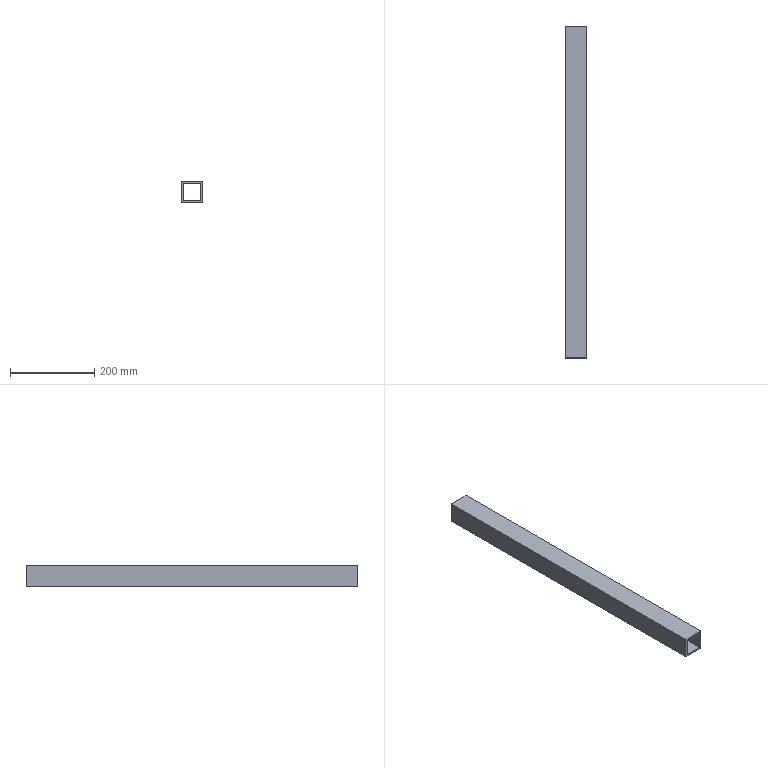Part | STEP file | PN_0082 pillar | 1 solid | 10 faces | box 50 x 790 x 50 mm | volume 581440 mm3 | plane 10
STEP:
#1=CARTESIAN_POINT('',(0.,0.,0.));
#2=DIRECTION('',(0.,0.,1.));
#3=DIRECTION('',(1.,0.,0.));
#4=AXIS2_PLACEMENT_3D('',#1,#2,#3);
#5=CARTESIAN_POINT('',(-25.,790.,-25.));
#6=VERTEX_POINT('',#5);
#7=CARTESIAN_POINT('',(-25.,790.,25.));
#8=VERTEX_POINT('',#7);
#9=CARTESIAN_POINT('',(-25.,790.,25.));
#10=DIRECTION('',(0.,0.,1.));
#11=VECTOR('',#10,1.);
#12=LINE('',#9,#11);
#13=CARTESIAN_POINT('',(0.,790.,0.));
#14=DIRECTION('',(0.,1.,0.));
#15=DIRECTION('',(0.,0.,1.));
#16=AXIS2_PLACEMENT_3D('',#13,#14,#15);
#17=PLANE('',#16);
#18=CARTESIAN_POINT('',(25.,-25.));
#19=DIRECTION('',(1.,0.));
#20=VECTOR('',#19,1.);
#21=LINE('',#18,#20);
#22=(GEOMETRIC_REPRESENTATION_CONTEXT(2)PARAMETRIC_REPRESENTATION_CONTEXT()REPRESENTATION_CONTEXT('',''));
#23=DEFINITIONAL_REPRESENTATION('',(#21),#22);
#24=PCURVE('',#17,#23);
#25=CARTESIAN_POINT('',(-25.,790.,25.));
#26=DIRECTION('',(1.,0.,0.));
#27=DIRECTION('',(0.,0.,-1.));
#28=AXIS2_PLACEMENT_3D('',#25,#26,#27);
#29=PLANE('',#28);
#30=CARTESIAN_POINT('',(0.,0.));
#31=DIRECTION('',(-1.,0.));
#32=VECTOR('',#31,1.);
#33=LINE('',#30,#32);
#34=(GEOMETRIC_REPRESENTATION_CONTEXT(2)PARAMETRIC_REPRESENTATION_CONTEXT()REPRESENTATION_CONTEXT('',''));
#35=DEFINITIONAL_REPRESENTATION('',(#33),#34);
#36=PCURVE('',#29,#35);
#37=SURFACE_CURVE('',#12,(#24,#36),.PCURVE_S1.);
#38=EDGE_CURVE('',#6,#8,#37,.T.);
#39=ORIENTED_EDGE('',*,*,#38,.T.);
#40=CARTESIAN_POINT('',(25.,790.,25.));
#41=VERTEX_POINT('',#40);
#42=CARTESIAN_POINT('',(25.,790.,25.));
#43=DIRECTION('',(1.,0.,0.));
#44=VECTOR('',#43,1.);
#45=LINE('',#42,#44);
#46=CARTESIAN_POINT('',(25.,25.));
#47=DIRECTION('',(0.,1.));
#48=VECTOR('',#47,1.);
#49=LINE('',#46,#48);
#50=(GEOMETRIC_REPRESENTATION_CONTEXT(2)PARAMETRIC_REPRESENTATION_CONTEXT()REPRESENTATION_CONTEXT('',''));
#51=DEFINITIONAL_REPRESENTATION('',(#49),#50);
#52=PCURVE('',#17,#51);
#53=CARTESIAN_POINT('',(25.,790.,25.));
#54=DIRECTION('',(0.,0.,-1.));
#55=DIRECTION('',(-1.,0.,0.));
#56=AXIS2_PLACEMENT_3D('',#53,#54,#55);
#57=PLANE('',#56);
#58=CARTESIAN_POINT('',(0.,0.));
#59=DIRECTION('',(-1.,0.));
#60=VECTOR('',#59,1.);
#61=LINE('',#58,#60);
#62=(GEOMETRIC_REPRESENTATION_CONTEXT(2)PARAMETRIC_REPRESENTATION_CONTEXT()REPRESENTATION_CONTEXT('',''));
#63=DEFINITIONAL_REPRESENTATION('',(#61),#62);
#64=PCURVE('',#57,#63);
#65=SURFACE_CURVE('',#45,(#52,#64),.PCURVE_S1.);
#66=EDGE_CURVE('',#8,#41,#65,.T.);
#67=ORIENTED_EDGE('',*,*,#66,.T.);
#68=CARTESIAN_POINT('',(25.,790.,-25.));
#69=VERTEX_POINT('',#68);
#70=CARTESIAN_POINT('',(25.,790.,25.));
#71=DIRECTION('',(0.,0.,-1.));
#72=VECTOR('',#71,1.);
#73=LINE('',#70,#72);
#74=CARTESIAN_POINT('',(25.,25.));
#75=DIRECTION('',(-1.,0.));
#76=VECTOR('',#75,1.);
#77=LINE('',#74,#76);
#78=(GEOMETRIC_REPRESENTATION_CONTEXT(2)PARAMETRIC_REPRESENTATION_CONTEXT()REPRESENTATION_CONTEXT('',''));
#79=DEFINITIONAL_REPRESENTATION('',(#77),#78);
#80=PCURVE('',#17,#79);
#81=CARTESIAN_POINT('',(25.,790.,25.));
#82=DIRECTION('',(-1.,0.,0.));
#83=DIRECTION('',(0.,0.,1.));
#84=AXIS2_PLACEMENT_3D('',#81,#82,#83);
#85=PLANE('',#84);
#86=CARTESIAN_POINT('',(0.,0.));
#87=DIRECTION('',(-1.,0.));
#88=VECTOR('',#87,1.);
#89=LINE('',#86,#88);
#90=(GEOMETRIC_REPRESENTATION_CONTEXT(2)PARAMETRIC_REPRESENTATION_CONTEXT()REPRESENTATION_CONTEXT('',''));
#91=DEFINITIONAL_REPRESENTATION('',(#89),#90);
#92=PCURVE('',#85,#91);
#93=SURFACE_CURVE('',#73,(#80,#92),.PCURVE_S1.);
#94=EDGE_CURVE('',#41,#69,#93,.T.);
#95=ORIENTED_EDGE('',*,*,#94,.T.);
#96=CARTESIAN_POINT('',(25.,790.,-25.));
#97=DIRECTION('',(-1.,0.,0.));
#98=VECTOR('',#97,1.);
#99=LINE('',#96,#98);
#100=CARTESIAN_POINT('',(-25.,25.));
#101=DIRECTION('',(0.,-1.));
#102=VECTOR('',#101,1.);
#103=LINE('',#100,#102);
#104=(GEOMETRIC_REPRESENTATION_CONTEXT(2)PARAMETRIC_REPRESENTATION_CONTEXT()REPRESENTATION_CONTEXT('',''));
#105=DEFINITIONAL_REPRESENTATION('',(#103),#104);
#106=PCURVE('',#17,#105);
#107=CARTESIAN_POINT('',(25.,790.,-25.));
#108=DIRECTION('',(0.,0.,1.));
#109=DIRECTION('',(1.,0.,0.));
#110=AXIS2_PLACEMENT_3D('',#107,#108,#109);
#111=PLANE('',#110);
#112=CARTESIAN_POINT('',(0.,0.));
#113=DIRECTION('',(-1.,0.));
#114=VECTOR('',#113,1.);
#115=LINE('',#112,#114);
#116=(GEOMETRIC_REPRESENTATION_CONTEXT(2)PARAMETRIC_REPRESENTATION_CONTEXT()REPRESENTATION_CONTEXT('',''));
#117=DEFINITIONAL_REPRESENTATION('',(#115),#116);
#118=PCURVE('',#111,#117);
#119=SURFACE_CURVE('',#99,(#106,#118),.PCURVE_S1.);
#120=EDGE_CURVE('',#69,#6,#119,.T.);
#121=ORIENTED_EDGE('',*,*,#120,.T.);
#122=EDGE_LOOP('',(#39,#67,#95,#121));
#123=FACE_BOUND('',#122,.T.);
#124=CARTESIAN_POINT('',(-21.,790.,21.));
#125=VERTEX_POINT('',#124);
#126=CARTESIAN_POINT('',(21.,790.,21.));
#127=VERTEX_POINT('',#126);
#128=CARTESIAN_POINT('',(21.,790.,21.));
#129=DIRECTION('',(1.,0.,0.));
#130=VECTOR('',#129,1.);
#131=LINE('',#128,#130);
#132=CARTESIAN_POINT('',(21.,21.));
#133=DIRECTION('',(0.,1.));
#134=VECTOR('',#133,1.);
#135=LINE('',#132,#134);
#136=(GEOMETRIC_REPRESENTATION_CONTEXT(2)PARAMETRIC_REPRESENTATION_CONTEXT()REPRESENTATION_CONTEXT('',''));
#137=DEFINITIONAL_REPRESENTATION('',(#135),#136);
#138=PCURVE('',#17,#137);
#139=CARTESIAN_POINT('',(21.,790.,21.));
#140=DIRECTION('',(0.,0.,-1.));
#141=DIRECTION('',(-1.,0.,0.));
#142=AXIS2_PLACEMENT_3D('',#139,#140,#141);
#143=PLANE('',#142);
#144=CARTESIAN_POINT('',(0.,0.));
#145=DIRECTION('',(-1.,0.));
#146=VECTOR('',#145,1.);
#147=LINE('',#144,#146);
#148=(GEOMETRIC_REPRESENTATION_CONTEXT(2)PARAMETRIC_REPRESENTATION_CONTEXT()REPRESENTATION_CONTEXT('',''));
#149=DEFINITIONAL_REPRESENTATION('',(#147),#148);
#150=PCURVE('',#143,#149);
#151=SURFACE_CURVE('',#131,(#138,#150),.PCURVE_S1.);
#152=EDGE_CURVE('',#125,#127,#151,.T.);
#153=ORIENTED_EDGE('',*,*,#152,.F.);
#154=CARTESIAN_POINT('',(-21.,790.,-21.));
#155=VERTEX_POINT('',#154);
#156=CARTESIAN_POINT('',(-21.,790.,21.));
#157=DIRECTION('',(0.,0.,1.));
#158=VECTOR('',#157,1.);
#159=LINE('',#156,#158);
#160=CARTESIAN_POINT('',(21.,-21.));
#161=DIRECTION('',(1.,0.));
#162=VECTOR('',#161,1.);
#163=LINE('',#160,#162);
#164=(GEOMETRIC_REPRESENTATION_CONTEXT(2)PARAMETRIC_REPRESENTATION_CONTEXT()REPRESENTATION_CONTEXT('',''));
#165=DEFINITIONAL_REPRESENTATION('',(#163),#164);
#166=PCURVE('',#17,#165);
#167=CARTESIAN_POINT('',(-21.,790.,21.));
#168=DIRECTION('',(1.,0.,0.));
#169=DIRECTION('',(0.,0.,-1.));
#170=AXIS2_PLACEMENT_3D('',#167,#168,#169);
#171=PLANE('',#170);
#172=CARTESIAN_POINT('',(0.,0.));
#173=DIRECTION('',(-1.,0.));
#174=VECTOR('',#173,1.);
#175=LINE('',#172,#174);
#176=(GEOMETRIC_REPRESENTATION_CONTEXT(2)PARAMETRIC_REPRESENTATION_CONTEXT()REPRESENTATION_CONTEXT('',''));
#177=DEFINITIONAL_REPRESENTATION('',(#175),#176);
#178=PCURVE('',#171,#177);
#179=SURFACE_CURVE('',#159,(#166,#178),.PCURVE_S1.);
#180=EDGE_CURVE('',#155,#125,#179,.T.);
#181=ORIENTED_EDGE('',*,*,#180,.F.);
#182=CARTESIAN_POINT('',(21.,790.,-21.));
#183=VERTEX_POINT('',#182);
#184=CARTESIAN_POINT('',(21.,790.,-21.));
#185=DIRECTION('',(-1.,0.,0.));
#186=VECTOR('',#185,1.);
#187=LINE('',#184,#186);
#188=CARTESIAN_POINT('',(-21.,21.));
#189=DIRECTION('',(0.,-1.));
#190=VECTOR('',#189,1.);
#191=LINE('',#188,#190);
#192=(GEOMETRIC_REPRESENTATION_CONTEXT(2)PARAMETRIC_REPRESENTATION_CONTEXT()REPRESENTATION_CONTEXT('',''));
#193=DEFINITIONAL_REPRESENTATION('',(#191),#192);
#194=PCURVE('',#17,#193);
#195=CARTESIAN_POINT('',(21.,790.,-21.));
#196=DIRECTION('',(0.,0.,1.));
#197=DIRECTION('',(1.,0.,0.));
#198=AXIS2_PLACEMENT_3D('',#195,#196,#197);
#199=PLANE('',#198);
#200=CARTESIAN_POINT('',(0.,0.));
#201=DIRECTION('',(-1.,0.));
#202=VECTOR('',#201,1.);
#203=LINE('',#200,#202);
#204=(GEOMETRIC_REPRESENTATION_CONTEXT(2)PARAMETRIC_REPRESENTATION_CONTEXT()REPRESENTATION_CONTEXT('',''));
#205=DEFINITIONAL_REPRESENTATION('',(#203),#204);
#206=PCURVE('',#199,#205);
#207=SURFACE_CURVE('',#187,(#194,#206),.PCURVE_S1.);
#208=EDGE_CURVE('',#183,#155,#207,.T.);
#209=ORIENTED_EDGE('',*,*,#208,.F.);
#210=CARTESIAN_POINT('',(21.,790.,21.));
#211=DIRECTION('',(0.,0.,-1.));
#212=VECTOR('',#211,1.);
#213=LINE('',#210,#212);
#214=CARTESIAN_POINT('',(21.,21.));
#215=DIRECTION('',(-1.,0.));
#216=VECTOR('',#215,1.);
#217=LINE('',#214,#216);
#218=(GEOMETRIC_REPRESENTATION_CONTEXT(2)PARAMETRIC_REPRESENTATION_CONTEXT()REPRESENTATION_CONTEXT('',''));
#219=DEFINITIONAL_REPRESENTATION('',(#217),#218);
#220=PCURVE('',#17,#219);
#221=CARTESIAN_POINT('',(21.,790.,21.));
#222=DIRECTION('',(-1.,0.,0.));
#223=DIRECTION('',(0.,0.,1.));
#224=AXIS2_PLACEMENT_3D('',#221,#222,#223);
#225=PLANE('',#224);
#226=CARTESIAN_POINT('',(0.,0.));
#227=DIRECTION('',(-1.,0.));
#228=VECTOR('',#227,1.);
#229=LINE('',#226,#228);
#230=(GEOMETRIC_REPRESENTATION_CONTEXT(2)PARAMETRIC_REPRESENTATION_CONTEXT()REPRESENTATION_CONTEXT('',''));
#231=DEFINITIONAL_REPRESENTATION('',(#229),#230);
#232=PCURVE('',#225,#231);
#233=SURFACE_CURVE('',#213,(#220,#232),.PCURVE_S1.);
#234=EDGE_CURVE('',#127,#183,#233,.T.);
#235=ORIENTED_EDGE('',*,*,#234,.F.);
#236=EDGE_LOOP('',(#153,#181,#209,#235));
#237=FACE_BOUND('',#236,.T.);
#238=ADVANCED_FACE('',(#123,#237),#17,.T.);
#239=CARTESIAN_POINT('',(-25.,0.,-25.));
#240=VERTEX_POINT('',#239);
#241=CARTESIAN_POINT('',(-25.,0.,25.));
#242=VERTEX_POINT('',#241);
#243=CARTESIAN_POINT('',(-25.,0.,25.));
#244=DIRECTION('',(0.,0.,1.));
#245=VECTOR('',#244,1.);
#246=LINE('',#243,#245);
#247=CARTESIAN_POINT('',(0.,0.,0.));
#248=DIRECTION('',(0.,1.,0.));
#249=DIRECTION('',(0.,0.,1.));
#250=AXIS2_PLACEMENT_3D('',#247,#248,#249);
#251=PLANE('',#250);
#252=CARTESIAN_POINT('',(25.,-25.));
#253=DIRECTION('',(1.,0.));
#254=VECTOR('',#253,1.);
#255=LINE('',#252,#254);
#256=(GEOMETRIC_REPRESENTATION_CONTEXT(2)PARAMETRIC_REPRESENTATION_CONTEXT()REPRESENTATION_CONTEXT('',''));
#257=DEFINITIONAL_REPRESENTATION('',(#255),#256);
#258=PCURVE('',#251,#257);
#259=CARTESIAN_POINT('',(0.,-790.));
#260=DIRECTION('',(-1.,0.));
#261=VECTOR('',#260,1.);
#262=LINE('',#259,#261);
#263=(GEOMETRIC_REPRESENTATION_CONTEXT(2)PARAMETRIC_REPRESENTATION_CONTEXT()REPRESENTATION_CONTEXT('',''));
#264=DEFINITIONAL_REPRESENTATION('',(#262),#263);
#265=PCURVE('',#29,#264);
#266=SURFACE_CURVE('',#246,(#258,#265),.PCURVE_S1.);
#267=EDGE_CURVE('',#240,#242,#266,.T.);
#268=ORIENTED_EDGE('',*,*,#267,.F.);
#269=CARTESIAN_POINT('',(25.,0.,-25.));
#270=VERTEX_POINT('',#269);
#271=CARTESIAN_POINT('',(25.,0.,-25.));
#272=DIRECTION('',(-1.,0.,0.));
#273=VECTOR('',#272,1.);
#274=LINE('',#271,#273);
#275=CARTESIAN_POINT('',(-25.,25.));
#276=DIRECTION('',(0.,-1.));
#277=VECTOR('',#276,1.);
#278=LINE('',#275,#277);
#279=(GEOMETRIC_REPRESENTATION_CONTEXT(2)PARAMETRIC_REPRESENTATION_CONTEXT()REPRESENTATION_CONTEXT('',''));
#280=DEFINITIONAL_REPRESENTATION('',(#278),#279);
#281=PCURVE('',#251,#280);
#282=CARTESIAN_POINT('',(0.,-790.));
#283=DIRECTION('',(-1.,0.));
#284=VECTOR('',#283,1.);
#285=LINE('',#282,#284);
#286=(GEOMETRIC_REPRESENTATION_CONTEXT(2)PARAMETRIC_REPRESENTATION_CONTEXT()REPRESENTATION_CONTEXT('',''));
#287=DEFINITIONAL_REPRESENTATION('',(#285),#286);
#288=PCURVE('',#111,#287);
#289=SURFACE_CURVE('',#274,(#281,#288),.PCURVE_S1.);
#290=EDGE_CURVE('',#270,#240,#289,.T.);
#291=ORIENTED_EDGE('',*,*,#290,.F.);
#292=CARTESIAN_POINT('',(25.,0.,25.));
#293=VERTEX_POINT('',#292);
#294=CARTESIAN_POINT('',(25.,0.,25.));
#295=DIRECTION('',(0.,0.,-1.));
#296=VECTOR('',#295,1.);
#297=LINE('',#294,#296);
#298=CARTESIAN_POINT('',(25.,25.));
#299=DIRECTION('',(-1.,0.));
#300=VECTOR('',#299,1.);
#301=LINE('',#298,#300);
#302=(GEOMETRIC_REPRESENTATION_CONTEXT(2)PARAMETRIC_REPRESENTATION_CONTEXT()REPRESENTATION_CONTEXT('',''));
#303=DEFINITIONAL_REPRESENTATION('',(#301),#302);
#304=PCURVE('',#251,#303);
#305=CARTESIAN_POINT('',(0.,-790.));
#306=DIRECTION('',(-1.,0.));
#307=VECTOR('',#306,1.);
#308=LINE('',#305,#307);
#309=(GEOMETRIC_REPRESENTATION_CONTEXT(2)PARAMETRIC_REPRESENTATION_CONTEXT()REPRESENTATION_CONTEXT('',''));
#310=DEFINITIONAL_REPRESENTATION('',(#308),#309);
#311=PCURVE('',#85,#310);
#312=SURFACE_CURVE('',#297,(#304,#311),.PCURVE_S1.);
#313=EDGE_CURVE('',#293,#270,#312,.T.);
#314=ORIENTED_EDGE('',*,*,#313,.F.);
#315=CARTESIAN_POINT('',(25.,0.,25.));
#316=DIRECTION('',(1.,0.,0.));
#317=VECTOR('',#316,1.);
#318=LINE('',#315,#317);
#319=CARTESIAN_POINT('',(25.,25.));
#320=DIRECTION('',(0.,1.));
#321=VECTOR('',#320,1.);
#322=LINE('',#319,#321);
#323=(GEOMETRIC_REPRESENTATION_CONTEXT(2)PARAMETRIC_REPRESENTATION_CONTEXT()REPRESENTATION_CONTEXT('',''));
#324=DEFINITIONAL_REPRESENTATION('',(#322),#323);
#325=PCURVE('',#251,#324);
#326=CARTESIAN_POINT('',(0.,-790.));
#327=DIRECTION('',(-1.,0.));
#328=VECTOR('',#327,1.);
#329=LINE('',#326,#328);
#330=(GEOMETRIC_REPRESENTATION_CONTEXT(2)PARAMETRIC_REPRESENTATION_CONTEXT()REPRESENTATION_CONTEXT('',''));
#331=DEFINITIONAL_REPRESENTATION('',(#329),#330);
#332=PCURVE('',#57,#331);
#333=SURFACE_CURVE('',#318,(#325,#332),.PCURVE_S1.);
#334=EDGE_CURVE('',#242,#293,#333,.T.);
#335=ORIENTED_EDGE('',*,*,#334,.F.);
#336=EDGE_LOOP('',(#268,#291,#314,#335));
#337=FACE_BOUND('',#336,.T.);
#338=CARTESIAN_POINT('',(-21.,0.,-21.));
#339=VERTEX_POINT('',#338);
#340=CARTESIAN_POINT('',(-21.,0.,21.));
#341=VERTEX_POINT('',#340);
#342=CARTESIAN_POINT('',(-21.,0.,21.));
#343=DIRECTION('',(0.,0.,1.));
#344=VECTOR('',#343,1.);
#345=LINE('',#342,#344);
#346=CARTESIAN_POINT('',(21.,-21.));
#347=DIRECTION('',(1.,0.));
#348=VECTOR('',#347,1.);
#349=LINE('',#346,#348);
#350=(GEOMETRIC_REPRESENTATION_CONTEXT(2)PARAMETRIC_REPRESENTATION_CONTEXT()REPRESENTATION_CONTEXT('',''));
#351=DEFINITIONAL_REPRESENTATION('',(#349),#350);
#352=PCURVE('',#251,#351);
#353=CARTESIAN_POINT('',(0.,-790.));
#354=DIRECTION('',(-1.,0.));
#355=VECTOR('',#354,1.);
#356=LINE('',#353,#355);
#357=(GEOMETRIC_REPRESENTATION_CONTEXT(2)PARAMETRIC_REPRESENTATION_CONTEXT()REPRESENTATION_CONTEXT('',''));
#358=DEFINITIONAL_REPRESENTATION('',(#356),#357);
#359=PCURVE('',#171,#358);
#360=SURFACE_CURVE('',#345,(#352,#359),.PCURVE_S1.);
#361=EDGE_CURVE('',#339,#341,#360,.T.);
#362=ORIENTED_EDGE('',*,*,#361,.T.);
#363=CARTESIAN_POINT('',(21.,0.,21.));
#364=VERTEX_POINT('',#363);
#365=CARTESIAN_POINT('',(21.,0.,21.));
#366=DIRECTION('',(1.,0.,0.));
#367=VECTOR('',#366,1.);
#368=LINE('',#365,#367);
#369=CARTESIAN_POINT('',(21.,21.));
#370=DIRECTION('',(0.,1.));
#371=VECTOR('',#370,1.);
#372=LINE('',#369,#371);
#373=(GEOMETRIC_REPRESENTATION_CONTEXT(2)PARAMETRIC_REPRESENTATION_CONTEXT()REPRESENTATION_CONTEXT('',''));
#374=DEFINITIONAL_REPRESENTATION('',(#372),#373);
#375=PCURVE('',#251,#374);
#376=CARTESIAN_POINT('',(0.,-790.));
#377=DIRECTION('',(-1.,0.));
#378=VECTOR('',#377,1.);
#379=LINE('',#376,#378);
#380=(GEOMETRIC_REPRESENTATION_CONTEXT(2)PARAMETRIC_REPRESENTATION_CONTEXT()REPRESENTATION_CONTEXT('',''));
#381=DEFINITIONAL_REPRESENTATION('',(#379),#380);
#382=PCURVE('',#143,#381);
#383=SURFACE_CURVE('',#368,(#375,#382),.PCURVE_S1.);
#384=EDGE_CURVE('',#341,#364,#383,.T.);
#385=ORIENTED_EDGE('',*,*,#384,.T.);
#386=CARTESIAN_POINT('',(21.,0.,-21.));
#387=VERTEX_POINT('',#386);
#388=CARTESIAN_POINT('',(21.,0.,21.));
#389=DIRECTION('',(0.,0.,-1.));
#390=VECTOR('',#389,1.);
#391=LINE('',#388,#390);
#392=CARTESIAN_POINT('',(21.,21.));
#393=DIRECTION('',(-1.,0.));
#394=VECTOR('',#393,1.);
#395=LINE('',#392,#394);
#396=(GEOMETRIC_REPRESENTATION_CONTEXT(2)PARAMETRIC_REPRESENTATION_CONTEXT()REPRESENTATION_CONTEXT('',''));
#397=DEFINITIONAL_REPRESENTATION('',(#395),#396);
#398=PCURVE('',#251,#397);
#399=CARTESIAN_POINT('',(0.,-790.));
#400=DIRECTION('',(-1.,0.));
#401=VECTOR('',#400,1.);
#402=LINE('',#399,#401);
#403=(GEOMETRIC_REPRESENTATION_CONTEXT(2)PARAMETRIC_REPRESENTATION_CONTEXT()REPRESENTATION_CONTEXT('',''));
#404=DEFINITIONAL_REPRESENTATION('',(#402),#403);
#405=PCURVE('',#225,#404);
#406=SURFACE_CURVE('',#391,(#398,#405),.PCURVE_S1.);
#407=EDGE_CURVE('',#364,#387,#406,.T.);
#408=ORIENTED_EDGE('',*,*,#407,.T.);
#409=CARTESIAN_POINT('',(21.,0.,-21.));
#410=DIRECTION('',(-1.,0.,0.));
#411=VECTOR('',#410,1.);
#412=LINE('',#409,#411);
#413=CARTESIAN_POINT('',(-21.,21.));
#414=DIRECTION('',(0.,-1.));
#415=VECTOR('',#414,1.);
#416=LINE('',#413,#415);
#417=(GEOMETRIC_REPRESENTATION_CONTEXT(2)PARAMETRIC_REPRESENTATION_CONTEXT()REPRESENTATION_CONTEXT('',''));
#418=DEFINITIONAL_REPRESENTATION('',(#416),#417);
#419=PCURVE('',#251,#418);
#420=CARTESIAN_POINT('',(0.,-790.));
#421=DIRECTION('',(-1.,0.));
#422=VECTOR('',#421,1.);
#423=LINE('',#420,#422);
#424=(GEOMETRIC_REPRESENTATION_CONTEXT(2)PARAMETRIC_REPRESENTATION_CONTEXT()REPRESENTATION_CONTEXT('',''));
#425=DEFINITIONAL_REPRESENTATION('',(#423),#424);
#426=PCURVE('',#199,#425);
#427=SURFACE_CURVE('',#412,(#419,#426),.PCURVE_S1.);
#428=EDGE_CURVE('',#387,#339,#427,.T.);
#429=ORIENTED_EDGE('',*,*,#428,.T.);
#430=EDGE_LOOP('',(#362,#385,#408,#429));
#431=FACE_BOUND('',#430,.T.);
#432=ADVANCED_FACE('',(#337,#431),#251,.F.);
#433=ORIENTED_EDGE('',*,*,#267,.T.);
#434=CARTESIAN_POINT('',(-25.,790.,25.));
#435=DIRECTION('',(0.,-1.,0.));
#436=VECTOR('',#435,1.);
#437=LINE('',#434,#436);
#438=CARTESIAN_POINT('',(0.,0.));
#439=DIRECTION('',(0.,-1.));
#440=VECTOR('',#439,1.);
#441=LINE('',#438,#440);
#442=(GEOMETRIC_REPRESENTATION_CONTEXT(2)PARAMETRIC_REPRESENTATION_CONTEXT()REPRESENTATION_CONTEXT('',''));
#443=DEFINITIONAL_REPRESENTATION('',(#441),#442);
#444=PCURVE('',#29,#443);
#445=CARTESIAN_POINT('',(50.,0.));
#446=DIRECTION('',(0.,-1.));
#447=VECTOR('',#446,1.);
#448=LINE('',#445,#447);
#449=(GEOMETRIC_REPRESENTATION_CONTEXT(2)PARAMETRIC_REPRESENTATION_CONTEXT()REPRESENTATION_CONTEXT('',''));
#450=DEFINITIONAL_REPRESENTATION('',(#448),#449);
#451=PCURVE('',#57,#450);
#452=SURFACE_CURVE('',#437,(#444,#451),.PCURVE_S1.);
#453=EDGE_CURVE('',#8,#242,#452,.T.);
#454=ORIENTED_EDGE('',*,*,#453,.F.);
#455=ORIENTED_EDGE('',*,*,#38,.F.);
#456=CARTESIAN_POINT('',(-25.,790.,-25.));
#457=DIRECTION('',(0.,-1.,0.));
#458=VECTOR('',#457,1.);
#459=LINE('',#456,#458);
#460=CARTESIAN_POINT('',(50.,0.));
#461=DIRECTION('',(0.,-1.));
#462=VECTOR('',#461,1.);
#463=LINE('',#460,#462);
#464=(GEOMETRIC_REPRESENTATION_CONTEXT(2)PARAMETRIC_REPRESENTATION_CONTEXT()REPRESENTATION_CONTEXT('',''));
#465=DEFINITIONAL_REPRESENTATION('',(#463),#464);
#466=PCURVE('',#29,#465);
#467=CARTESIAN_POINT('',(-50.,0.));
#468=DIRECTION('',(0.,-1.));
#469=VECTOR('',#468,1.);
#470=LINE('',#467,#469);
#471=(GEOMETRIC_REPRESENTATION_CONTEXT(2)PARAMETRIC_REPRESENTATION_CONTEXT()REPRESENTATION_CONTEXT('',''));
#472=DEFINITIONAL_REPRESENTATION('',(#470),#471);
#473=PCURVE('',#111,#472);
#474=SURFACE_CURVE('',#459,(#466,#473),.PCURVE_S1.);
#475=EDGE_CURVE('',#6,#240,#474,.T.);
#476=ORIENTED_EDGE('',*,*,#475,.T.);
#477=EDGE_LOOP('',(#433,#454,#455,#476));
#478=FACE_BOUND('',#477,.T.);
#479=ADVANCED_FACE('',(#478),#29,.F.);
#480=ORIENTED_EDGE('',*,*,#334,.T.);
#481=CARTESIAN_POINT('',(25.,790.,25.));
#482=DIRECTION('',(0.,-1.,0.));
#483=VECTOR('',#482,1.);
#484=LINE('',#481,#483);
#485=CARTESIAN_POINT('',(0.,0.));
#486=DIRECTION('',(0.,-1.));
#487=VECTOR('',#486,1.);
#488=LINE('',#485,#487);
#489=(GEOMETRIC_REPRESENTATION_CONTEXT(2)PARAMETRIC_REPRESENTATION_CONTEXT()REPRESENTATION_CONTEXT('',''));
#490=DEFINITIONAL_REPRESENTATION('',(#488),#489);
#491=PCURVE('',#57,#490);
#492=CARTESIAN_POINT('',(0.,0.));
#493=DIRECTION('',(0.,-1.));
#494=VECTOR('',#493,1.);
#495=LINE('',#492,#494);
#496=(GEOMETRIC_REPRESENTATION_CONTEXT(2)PARAMETRIC_REPRESENTATION_CONTEXT()REPRESENTATION_CONTEXT('',''));
#497=DEFINITIONAL_REPRESENTATION('',(#495),#496);
#498=PCURVE('',#85,#497);
#499=SURFACE_CURVE('',#484,(#491,#498),.PCURVE_S1.);
#500=EDGE_CURVE('',#41,#293,#499,.T.);
#501=ORIENTED_EDGE('',*,*,#500,.F.);
#502=ORIENTED_EDGE('',*,*,#66,.F.);
#503=ORIENTED_EDGE('',*,*,#453,.T.);
#504=EDGE_LOOP('',(#480,#501,#502,#503));
#505=FACE_BOUND('',#504,.T.);
#506=ADVANCED_FACE('',(#505),#57,.F.);
#507=ORIENTED_EDGE('',*,*,#313,.T.);
#508=CARTESIAN_POINT('',(25.,790.,-25.));
#509=DIRECTION('',(0.,-1.,0.));
#510=VECTOR('',#509,1.);
#511=LINE('',#508,#510);
#512=CARTESIAN_POINT('',(-50.,0.));
#513=DIRECTION('',(0.,-1.));
#514=VECTOR('',#513,1.);
#515=LINE('',#512,#514);
#516=(GEOMETRIC_REPRESENTATION_CONTEXT(2)PARAMETRIC_REPRESENTATION_CONTEXT()REPRESENTATION_CONTEXT('',''));
#517=DEFINITIONAL_REPRESENTATION('',(#515),#516);
#518=PCURVE('',#85,#517);
#519=CARTESIAN_POINT('',(0.,0.));
#520=DIRECTION('',(0.,-1.));
#521=VECTOR('',#520,1.);
#522=LINE('',#519,#521);
#523=(GEOMETRIC_REPRESENTATION_CONTEXT(2)PARAMETRIC_REPRESENTATION_CONTEXT()REPRESENTATION_CONTEXT('',''));
#524=DEFINITIONAL_REPRESENTATION('',(#522),#523);
#525=PCURVE('',#111,#524);
#526=SURFACE_CURVE('',#511,(#518,#525),.PCURVE_S1.);
#527=EDGE_CURVE('',#69,#270,#526,.T.);
#528=ORIENTED_EDGE('',*,*,#527,.F.);
#529=ORIENTED_EDGE('',*,*,#94,.F.);
#530=ORIENTED_EDGE('',*,*,#500,.T.);
#531=EDGE_LOOP('',(#507,#528,#529,#530));
#532=FACE_BOUND('',#531,.T.);
#533=ADVANCED_FACE('',(#532),#85,.F.);
#534=ORIENTED_EDGE('',*,*,#290,.T.);
#535=ORIENTED_EDGE('',*,*,#475,.F.);
#536=ORIENTED_EDGE('',*,*,#120,.F.);
#537=ORIENTED_EDGE('',*,*,#527,.T.);
#538=EDGE_LOOP('',(#534,#535,#536,#537));
#539=FACE_BOUND('',#538,.T.);
#540=ADVANCED_FACE('',(#539),#111,.F.);
#541=ORIENTED_EDGE('',*,*,#361,.F.);
#542=CARTESIAN_POINT('',(-21.,790.,-21.));
#543=DIRECTION('',(0.,-1.,0.));
#544=VECTOR('',#543,1.);
#545=LINE('',#542,#544);
#546=CARTESIAN_POINT('',(42.,0.));
#547=DIRECTION('',(0.,-1.));
#548=VECTOR('',#547,1.);
#549=LINE('',#546,#548);
#550=(GEOMETRIC_REPRESENTATION_CONTEXT(2)PARAMETRIC_REPRESENTATION_CONTEXT()REPRESENTATION_CONTEXT('',''));
#551=DEFINITIONAL_REPRESENTATION('',(#549),#550);
#552=PCURVE('',#171,#551);
#553=CARTESIAN_POINT('',(-42.,0.));
#554=DIRECTION('',(0.,-1.));
#555=VECTOR('',#554,1.);
#556=LINE('',#553,#555);
#557=(GEOMETRIC_REPRESENTATION_CONTEXT(2)PARAMETRIC_REPRESENTATION_CONTEXT()REPRESENTATION_CONTEXT('',''));
#558=DEFINITIONAL_REPRESENTATION('',(#556),#557);
#559=PCURVE('',#199,#558);
#560=SURFACE_CURVE('',#545,(#552,#559),.PCURVE_S1.);
#561=EDGE_CURVE('',#155,#339,#560,.T.);
#562=ORIENTED_EDGE('',*,*,#561,.F.);
#563=ORIENTED_EDGE('',*,*,#180,.T.);
#564=CARTESIAN_POINT('',(-21.,790.,21.));
#565=DIRECTION('',(0.,-1.,0.));
#566=VECTOR('',#565,1.);
#567=LINE('',#564,#566);
#568=CARTESIAN_POINT('',(0.,0.));
#569=DIRECTION('',(0.,-1.));
#570=VECTOR('',#569,1.);
#571=LINE('',#568,#570);
#572=(GEOMETRIC_REPRESENTATION_CONTEXT(2)PARAMETRIC_REPRESENTATION_CONTEXT()REPRESENTATION_CONTEXT('',''));
#573=DEFINITIONAL_REPRESENTATION('',(#571),#572);
#574=PCURVE('',#171,#573);
#575=CARTESIAN_POINT('',(42.,0.));
#576=DIRECTION('',(0.,-1.));
#577=VECTOR('',#576,1.);
#578=LINE('',#575,#577);
#579=(GEOMETRIC_REPRESENTATION_CONTEXT(2)PARAMETRIC_REPRESENTATION_CONTEXT()REPRESENTATION_CONTEXT('',''));
#580=DEFINITIONAL_REPRESENTATION('',(#578),#579);
#581=PCURVE('',#143,#580);
#582=SURFACE_CURVE('',#567,(#574,#581),.PCURVE_S1.);
#583=EDGE_CURVE('',#125,#341,#582,.T.);
#584=ORIENTED_EDGE('',*,*,#583,.T.);
#585=EDGE_LOOP('',(#541,#562,#563,#584));
#586=FACE_BOUND('',#585,.T.);
#587=ADVANCED_FACE('',(#586),#171,.T.);
#588=ORIENTED_EDGE('',*,*,#384,.F.);
#589=ORIENTED_EDGE('',*,*,#583,.F.);
#590=ORIENTED_EDGE('',*,*,#152,.T.);
#591=CARTESIAN_POINT('',(21.,790.,21.));
#592=DIRECTION('',(0.,-1.,0.));
#593=VECTOR('',#592,1.);
#594=LINE('',#591,#593);
#595=CARTESIAN_POINT('',(0.,0.));
#596=DIRECTION('',(0.,-1.));
#597=VECTOR('',#596,1.);
#598=LINE('',#595,#597);
#599=(GEOMETRIC_REPRESENTATION_CONTEXT(2)PARAMETRIC_REPRESENTATION_CONTEXT()REPRESENTATION_CONTEXT('',''));
#600=DEFINITIONAL_REPRESENTATION('',(#598),#599);
#601=PCURVE('',#143,#600);
#602=CARTESIAN_POINT('',(0.,0.));
#603=DIRECTION('',(0.,-1.));
#604=VECTOR('',#603,1.);
#605=LINE('',#602,#604);
#606=(GEOMETRIC_REPRESENTATION_CONTEXT(2)PARAMETRIC_REPRESENTATION_CONTEXT()REPRESENTATION_CONTEXT('',''));
#607=DEFINITIONAL_REPRESENTATION('',(#605),#606);
#608=PCURVE('',#225,#607);
#609=SURFACE_CURVE('',#594,(#601,#608),.PCURVE_S1.);
#610=EDGE_CURVE('',#127,#364,#609,.T.);
#611=ORIENTED_EDGE('',*,*,#610,.T.);
#612=EDGE_LOOP('',(#588,#589,#590,#611));
#613=FACE_BOUND('',#612,.T.);
#614=ADVANCED_FACE('',(#613),#143,.T.);
#615=ORIENTED_EDGE('',*,*,#407,.F.);
#616=ORIENTED_EDGE('',*,*,#610,.F.);
#617=ORIENTED_EDGE('',*,*,#234,.T.);
#618=CARTESIAN_POINT('',(21.,790.,-21.));
#619=DIRECTION('',(0.,-1.,0.));
#620=VECTOR('',#619,1.);
#621=LINE('',#618,#620);
#622=CARTESIAN_POINT('',(-42.,0.));
#623=DIRECTION('',(0.,-1.));
#624=VECTOR('',#623,1.);
#625=LINE('',#622,#624);
#626=(GEOMETRIC_REPRESENTATION_CONTEXT(2)PARAMETRIC_REPRESENTATION_CONTEXT()REPRESENTATION_CONTEXT('',''));
#627=DEFINITIONAL_REPRESENTATION('',(#625),#626);
#628=PCURVE('',#225,#627);
#629=CARTESIAN_POINT('',(0.,0.));
#630=DIRECTION('',(0.,-1.));
#631=VECTOR('',#630,1.);
#632=LINE('',#629,#631);
#633=(GEOMETRIC_REPRESENTATION_CONTEXT(2)PARAMETRIC_REPRESENTATION_CONTEXT()REPRESENTATION_CONTEXT('',''));
#634=DEFINITIONAL_REPRESENTATION('',(#632),#633);
#635=PCURVE('',#199,#634);
#636=SURFACE_CURVE('',#621,(#628,#635),.PCURVE_S1.);
#637=EDGE_CURVE('',#183,#387,#636,.T.);
#638=ORIENTED_EDGE('',*,*,#637,.T.);
#639=EDGE_LOOP('',(#615,#616,#617,#638));
#640=FACE_BOUND('',#639,.T.);
#641=ADVANCED_FACE('',(#640),#225,.T.);
#642=ORIENTED_EDGE('',*,*,#428,.F.);
#643=ORIENTED_EDGE('',*,*,#637,.F.);
#644=ORIENTED_EDGE('',*,*,#208,.T.);
#645=ORIENTED_EDGE('',*,*,#561,.T.);
#646=EDGE_LOOP('',(#642,#643,#644,#645));
#647=FACE_BOUND('',#646,.T.);
#648=ADVANCED_FACE('',(#647),#199,.T.);
#649=CLOSED_SHELL('',(#238,#432,#479,#506,#533,#540,#587,#614,#641,#648));
#650=MANIFOLD_SOLID_BREP('',#649);
#651=(LENGTH_UNIT()NAMED_UNIT(*)SI_UNIT(.MILLI.,.METRE.));
#652=UNCERTAINTY_MEASURE_WITH_UNIT(LENGTH_MEASURE(0.0000001),#651,'','');
#653=(NAMED_UNIT(*)PLANE_ANGLE_UNIT()SI_UNIT($,.RADIAN.));
#654=(NAMED_UNIT(*)SI_UNIT($,.STERADIAN.)SOLID_ANGLE_UNIT());
#655=(GEOMETRIC_REPRESENTATION_CONTEXT(3)GLOBAL_UNCERTAINTY_ASSIGNED_CONTEXT((#652))GLOBAL_UNIT_ASSIGNED_CONTEXT((#651,#653,#654))REPRESENTATION_CONTEXT('',''));
#656=ADVANCED_BREP_SHAPE_REPRESENTATION('',(#4,#650),#655);